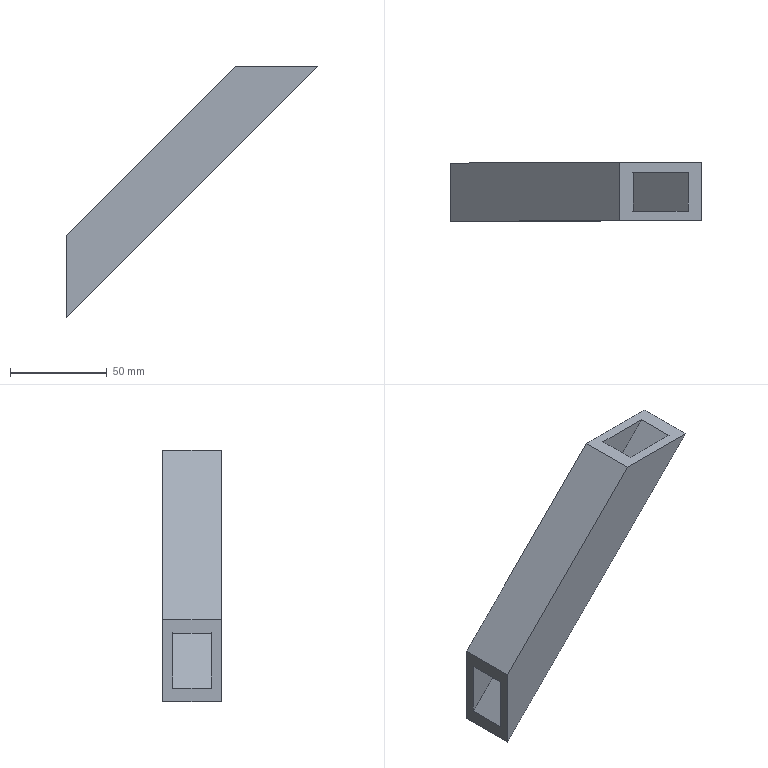Part | NX | features solid 2 | 1 solid | 10 faces | box 130 x 30 x 130 mm | volume 76924 mm3 | plane 10
STEP:
#1=CARTESIAN_POINT('',(205.,215.,-137.574));
#2=VERTEX_POINT('',#1);
#3=CARTESIAN_POINT('',(292.574,215.,-50.));
#4=VERTEX_POINT('',#3);
#5=CARTESIAN_POINT('',(235.,215.,-107.574));
#6=DIRECTION('',(0.7071,0.,0.7071));
#7=VECTOR('',#6,1000.);
#8=LINE('',#5,#7);
#9=EDGE_CURVE('',#2,#4,#8,.T.);
#10=ORIENTED_EDGE('',*,*,#9,.T.);
#11=CARTESIAN_POINT('',(292.574,245.,-50.));
#12=VERTEX_POINT('',#11);
#13=CARTESIAN_POINT('',(292.574,245.,-50.));
#14=DIRECTION('',(0.,1.,0.));
#15=VECTOR('',#14,1000.);
#16=LINE('',#13,#15);
#17=EDGE_CURVE('',#12,#4,#16,.F.);
#18=ORIENTED_EDGE('',*,*,#17,.F.);
#19=CARTESIAN_POINT('',(205.,245.,-137.574));
#20=VERTEX_POINT('',#19);
#21=CARTESIAN_POINT('',(235.,245.,-107.574));
#22=DIRECTION('',(0.7071,0.,0.7071));
#23=VECTOR('',#22,1000.);
#24=LINE('',#21,#23);
#25=EDGE_CURVE('',#20,#12,#24,.T.);
#26=ORIENTED_EDGE('',*,*,#25,.F.);
#27=CARTESIAN_POINT('',(205.,245.,-137.574));
#28=DIRECTION('',(0.,1.,0.));
#29=VECTOR('',#28,1000.);
#30=LINE('',#27,#29);
#31=EDGE_CURVE('',#2,#20,#30,.T.);
#32=ORIENTED_EDGE('',*,*,#31,.F.);
#33=EDGE_LOOP('',(#10,#18,#26,#32));
#34=FACE_BOUND('',#33,.T.);
#35=CARTESIAN_POINT('',(235.,245.,-107.574));
#36=DIRECTION('',(0.7071,0.,-0.7071));
#37=DIRECTION('',(0.7071,0.,0.7071));
#38=AXIS2_PLACEMENT_3D('',#35,#36,#37);
#39=PLANE('',#38);
#40=ADVANCED_FACE('',(#34),#39,.F.);
#41=CARTESIAN_POINT('',(205.,215.,-180.));
#42=VERTEX_POINT('',#41);
#43=CARTESIAN_POINT('',(205.,245.,-180.));
#44=VERTEX_POINT('',#43);
#45=CARTESIAN_POINT('',(205.,245.,-180.));
#46=DIRECTION('',(0.,1.,0.));
#47=VECTOR('',#46,1000.);
#48=LINE('',#45,#47);
#49=EDGE_CURVE('',#42,#44,#48,.T.);
#50=ORIENTED_EDGE('',*,*,#49,.T.);
#51=CARTESIAN_POINT('',(335.,245.,-50.));
#52=VERTEX_POINT('',#51);
#53=CARTESIAN_POINT('',(256.213,245.,-128.787));
#54=DIRECTION('',(0.7071,0.,0.7071));
#55=VECTOR('',#54,1000.);
#56=LINE('',#53,#55);
#57=EDGE_CURVE('',#44,#52,#56,.T.);
#58=ORIENTED_EDGE('',*,*,#57,.T.);
#59=CARTESIAN_POINT('',(335.,215.,-50.));
#60=VERTEX_POINT('',#59);
#61=CARTESIAN_POINT('',(335.,245.,-50.));
#62=DIRECTION('',(0.,1.,0.));
#63=VECTOR('',#62,1000.);
#64=LINE('',#61,#63);
#65=EDGE_CURVE('',#52,#60,#64,.F.);
#66=ORIENTED_EDGE('',*,*,#65,.T.);
#67=CARTESIAN_POINT('',(256.213,215.,-128.787));
#68=DIRECTION('',(0.7071,0.,0.7071));
#69=VECTOR('',#68,1000.);
#70=LINE('',#67,#69);
#71=EDGE_CURVE('',#42,#60,#70,.T.);
#72=ORIENTED_EDGE('',*,*,#71,.F.);
#73=EDGE_LOOP('',(#50,#58,#66,#72));
#74=FACE_BOUND('',#73,.T.);
#75=CARTESIAN_POINT('',(256.213,245.,-128.787));
#76=DIRECTION('',(0.7071,0.,-0.7071));
#77=DIRECTION('',(0.7071,0.,0.7071));
#78=AXIS2_PLACEMENT_3D('',#75,#76,#77);
#79=PLANE('',#78);
#80=ADVANCED_FACE('',(#74),#79,.T.);
#81=ORIENTED_EDGE('',*,*,#25,.T.);
#82=CARTESIAN_POINT('',(235.,245.,-50.));
#83=DIRECTION('',(1.,0.,0.));
#84=VECTOR('',#83,1000.);
#85=LINE('',#82,#84);
#86=EDGE_CURVE('',#52,#12,#85,.F.);
#87=ORIENTED_EDGE('',*,*,#86,.F.);
#88=ORIENTED_EDGE('',*,*,#57,.F.);
#89=CARTESIAN_POINT('',(205.,245.,-107.574));
#90=DIRECTION('',(0.,0.,-1.));
#91=VECTOR('',#90,1000.);
#92=LINE('',#89,#91);
#93=EDGE_CURVE('',#20,#44,#92,.T.);
#94=ORIENTED_EDGE('',*,*,#93,.F.);
#95=EDGE_LOOP('',(#81,#87,#88,#94));
#96=FACE_BOUND('',#95,.T.);
#97=CARTESIAN_POINT('',(235.,245.,-107.574));
#98=DIRECTION('',(0.,-1.,0.));
#99=DIRECTION('',(0.7071,0.,0.7071));
#100=AXIS2_PLACEMENT_3D('',#97,#98,#99);
#101=PLANE('',#100);
#102=ADVANCED_FACE('',(#96),#101,.F.);
#103=ORIENTED_EDGE('',*,*,#71,.T.);
#104=CARTESIAN_POINT('',(235.,215.,-50.));
#105=DIRECTION('',(1.,0.,0.));
#106=VECTOR('',#105,1000.);
#107=LINE('',#104,#106);
#108=EDGE_CURVE('',#4,#60,#107,.T.);
#109=ORIENTED_EDGE('',*,*,#108,.F.);
#110=ORIENTED_EDGE('',*,*,#9,.F.);
#111=CARTESIAN_POINT('',(205.,215.,-107.574));
#112=DIRECTION('',(0.,0.,-1.));
#113=VECTOR('',#112,1000.);
#114=LINE('',#111,#113);
#115=EDGE_CURVE('',#42,#2,#114,.F.);
#116=ORIENTED_EDGE('',*,*,#115,.F.);
#117=EDGE_LOOP('',(#103,#109,#110,#116));
#118=FACE_BOUND('',#117,.T.);
#119=CARTESIAN_POINT('',(235.,215.,-107.574));
#120=DIRECTION('',(0.,-1.,0.));
#121=DIRECTION('',(0.7071,0.,0.7071));
#122=AXIS2_PLACEMENT_3D('',#119,#120,#121);
#123=PLANE('',#122);
#124=ADVANCED_FACE('',(#118),#123,.T.);
#125=CARTESIAN_POINT('',(205.,220.,-144.645));
#126=VERTEX_POINT('',#125);
#127=CARTESIAN_POINT('',(205.,240.,-144.645));
#128=VERTEX_POINT('',#127);
#129=CARTESIAN_POINT('',(205.,245.,-144.645));
#130=DIRECTION('',(0.,1.,0.));
#131=VECTOR('',#130,1000.);
#132=LINE('',#129,#131);
#133=EDGE_CURVE('',#126,#128,#132,.T.);
#134=ORIENTED_EDGE('',*,*,#133,.T.);
#135=CARTESIAN_POINT('',(299.645,240.,-50.));
#136=VERTEX_POINT('',#135);
#137=CARTESIAN_POINT('',(238.536,240.,-111.109));
#138=DIRECTION('',(0.7071,0.,0.7071));
#139=VECTOR('',#138,1000.);
#140=LINE('',#137,#139);
#141=EDGE_CURVE('',#128,#136,#140,.T.);
#142=ORIENTED_EDGE('',*,*,#141,.T.);
#143=CARTESIAN_POINT('',(299.645,220.,-50.));
#144=VERTEX_POINT('',#143);
#145=CARTESIAN_POINT('',(299.645,245.,-50.));
#146=DIRECTION('',(0.,1.,0.));
#147=VECTOR('',#146,1000.);
#148=LINE('',#145,#147);
#149=EDGE_CURVE('',#136,#144,#148,.F.);
#150=ORIENTED_EDGE('',*,*,#149,.T.);
#151=CARTESIAN_POINT('',(238.536,220.,-111.109));
#152=DIRECTION('',(-0.7071,0.,-0.7071));
#153=VECTOR('',#152,1000.);
#154=LINE('',#151,#153);
#155=EDGE_CURVE('',#126,#144,#154,.F.);
#156=ORIENTED_EDGE('',*,*,#155,.F.);
#157=EDGE_LOOP('',(#134,#142,#150,#156));
#158=FACE_BOUND('',#157,.T.);
#159=CARTESIAN_POINT('',(238.536,245.,-111.109));
#160=DIRECTION('',(0.7071,0.,-0.7071));
#161=DIRECTION('',(0.7071,0.,0.7071));
#162=AXIS2_PLACEMENT_3D('',#159,#160,#161);
#163=PLANE('',#162);
#164=ADVANCED_FACE('',(#158),#163,.T.);
#165=CARTESIAN_POINT('',(205.,220.,-172.929));
#166=VERTEX_POINT('',#165);
#167=CARTESIAN_POINT('',(327.929,220.,-50.));
#168=VERTEX_POINT('',#167);
#169=CARTESIAN_POINT('',(252.678,220.,-125.251));
#170=DIRECTION('',(-0.7071,0.,-0.7071));
#171=VECTOR('',#170,1000.);
#172=LINE('',#169,#171);
#173=EDGE_CURVE('',#166,#168,#172,.F.);
#174=ORIENTED_EDGE('',*,*,#173,.T.);
#175=CARTESIAN_POINT('',(327.929,240.,-50.));
#176=VERTEX_POINT('',#175);
#177=CARTESIAN_POINT('',(327.929,245.,-50.));
#178=DIRECTION('',(0.,1.,0.));
#179=VECTOR('',#178,1000.);
#180=LINE('',#177,#179);
#181=EDGE_CURVE('',#176,#168,#180,.F.);
#182=ORIENTED_EDGE('',*,*,#181,.F.);
#183=CARTESIAN_POINT('',(205.,240.,-172.929));
#184=VERTEX_POINT('',#183);
#185=CARTESIAN_POINT('',(252.678,240.,-125.251));
#186=DIRECTION('',(0.7071,0.,0.7071));
#187=VECTOR('',#186,1000.);
#188=LINE('',#185,#187);
#189=EDGE_CURVE('',#184,#176,#188,.T.);
#190=ORIENTED_EDGE('',*,*,#189,.F.);
#191=CARTESIAN_POINT('',(205.,245.,-172.929));
#192=DIRECTION('',(0.,1.,0.));
#193=VECTOR('',#192,1000.);
#194=LINE('',#191,#193);
#195=EDGE_CURVE('',#166,#184,#194,.T.);
#196=ORIENTED_EDGE('',*,*,#195,.F.);
#197=EDGE_LOOP('',(#174,#182,#190,#196));
#198=FACE_BOUND('',#197,.T.);
#199=CARTESIAN_POINT('',(252.678,245.,-125.251));
#200=DIRECTION('',(0.7071,0.,-0.7071));
#201=DIRECTION('',(0.7071,0.,0.7071));
#202=AXIS2_PLACEMENT_3D('',#199,#200,#201);
#203=PLANE('',#202);
#204=ADVANCED_FACE('',(#198),#203,.F.);
#205=CARTESIAN_POINT('',(205.,240.,-107.574));
#206=DIRECTION('',(0.,0.,-1.));
#207=VECTOR('',#206,1000.);
#208=LINE('',#205,#207);
#209=EDGE_CURVE('',#128,#184,#208,.T.);
#210=ORIENTED_EDGE('',*,*,#209,.T.);
#211=ORIENTED_EDGE('',*,*,#189,.T.);
#212=CARTESIAN_POINT('',(235.,240.,-50.));
#213=DIRECTION('',(1.,0.,0.));
#214=VECTOR('',#213,1000.);
#215=LINE('',#212,#214);
#216=EDGE_CURVE('',#176,#136,#215,.F.);
#217=ORIENTED_EDGE('',*,*,#216,.T.);
#218=ORIENTED_EDGE('',*,*,#141,.F.);
#219=EDGE_LOOP('',(#210,#211,#217,#218));
#220=FACE_BOUND('',#219,.T.);
#221=CARTESIAN_POINT('',(235.,240.,-107.574));
#222=DIRECTION('',(0.,-1.,0.));
#223=DIRECTION('',(0.7071,0.,0.7071));
#224=AXIS2_PLACEMENT_3D('',#221,#222,#223);
#225=PLANE('',#224);
#226=ADVANCED_FACE('',(#220),#225,.T.);
#227=CARTESIAN_POINT('',(205.,220.,-107.574));
#228=DIRECTION('',(0.,0.,-1.));
#229=VECTOR('',#228,1000.);
#230=LINE('',#227,#229);
#231=EDGE_CURVE('',#166,#126,#230,.F.);
#232=ORIENTED_EDGE('',*,*,#231,.T.);
#233=ORIENTED_EDGE('',*,*,#155,.T.);
#234=CARTESIAN_POINT('',(235.,220.,-50.));
#235=DIRECTION('',(1.,0.,0.));
#236=VECTOR('',#235,1000.);
#237=LINE('',#234,#236);
#238=EDGE_CURVE('',#144,#168,#237,.T.);
#239=ORIENTED_EDGE('',*,*,#238,.T.);
#240=ORIENTED_EDGE('',*,*,#173,.F.);
#241=EDGE_LOOP('',(#232,#233,#239,#240));
#242=FACE_BOUND('',#241,.T.);
#243=CARTESIAN_POINT('',(235.,220.,-107.574));
#244=DIRECTION('',(0.,-1.,0.));
#245=DIRECTION('',(0.7071,0.,0.7071));
#246=AXIS2_PLACEMENT_3D('',#243,#244,#245);
#247=PLANE('',#246);
#248=ADVANCED_FACE('',(#242),#247,.F.);
#249=ORIENTED_EDGE('',*,*,#149,.F.);
#250=ORIENTED_EDGE('',*,*,#216,.F.);
#251=ORIENTED_EDGE('',*,*,#181,.T.);
#252=ORIENTED_EDGE('',*,*,#238,.F.);
#253=EDGE_LOOP('',(#249,#250,#251,#252));
#254=FACE_BOUND('',#253,.T.);
#255=ORIENTED_EDGE('',*,*,#86,.T.);
#256=ORIENTED_EDGE('',*,*,#17,.T.);
#257=ORIENTED_EDGE('',*,*,#108,.T.);
#258=ORIENTED_EDGE('',*,*,#65,.F.);
#259=EDGE_LOOP('',(#255,#256,#257,#258));
#260=FACE_BOUND('',#259,.T.);
#261=CARTESIAN_POINT('',(205.,245.,-50.));
#262=DIRECTION('',(0.,0.,1.));
#263=DIRECTION('',(0.,-1.,0.));
#264=AXIS2_PLACEMENT_3D('',#261,#262,#263);
#265=PLANE('',#264);
#266=ADVANCED_FACE('',(#254,#260),#265,.T.);
#267=ORIENTED_EDGE('',*,*,#209,.F.);
#268=ORIENTED_EDGE('',*,*,#133,.F.);
#269=ORIENTED_EDGE('',*,*,#231,.F.);
#270=ORIENTED_EDGE('',*,*,#195,.T.);
#271=EDGE_LOOP('',(#267,#268,#269,#270));
#272=FACE_BOUND('',#271,.T.);
#273=ORIENTED_EDGE('',*,*,#31,.T.);
#274=ORIENTED_EDGE('',*,*,#93,.T.);
#275=ORIENTED_EDGE('',*,*,#49,.F.);
#276=ORIENTED_EDGE('',*,*,#115,.T.);
#277=EDGE_LOOP('',(#273,#274,#275,#276));
#278=FACE_BOUND('',#277,.T.);
#279=CARTESIAN_POINT('',(205.,295.,-180.));
#280=DIRECTION('',(1.,0.,0.));
#281=DIRECTION('',(0.,0.,1.));
#282=AXIS2_PLACEMENT_3D('',#279,#280,#281);
#283=PLANE('',#282);
#284=ADVANCED_FACE('',(#272,#278),#283,.F.);
#285=CLOSED_SHELL('',(#40,#80,#102,#124,#164,#204,#226,#248,#266,#284));
#286=MANIFOLD_SOLID_BREP('',#285);
#287=(LENGTH_UNIT()NAMED_UNIT(*)SI_UNIT(.MILLI.,.METRE.));
#288=UNCERTAINTY_MEASURE_WITH_UNIT(LENGTH_MEASURE(0.00001),#287,'','');
#289=(NAMED_UNIT(*)PLANE_ANGLE_UNIT()SI_UNIT($,.RADIAN.));
#290=(NAMED_UNIT(*)SI_UNIT($,.STERADIAN.)SOLID_ANGLE_UNIT());
#291=(GEOMETRIC_REPRESENTATION_CONTEXT(3)GLOBAL_UNCERTAINTY_ASSIGNED_CONTEXT((#288))GLOBAL_UNIT_ASSIGNED_CONTEXT((#287,#289,#290))REPRESENTATION_CONTEXT('',''));
#292=ADVANCED_BREP_SHAPE_REPRESENTATION('',(#286),#291);